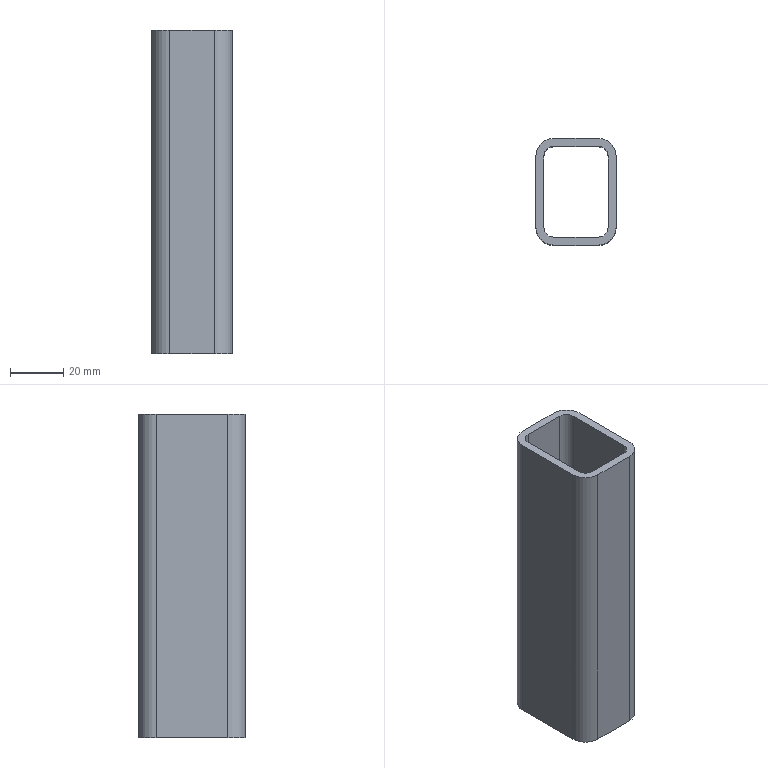Part | STEP file | DIN EN 10305-5 40 x 30 x 3 1785429634942 | 1 solid | 18 faces | box 30 x 40 x 121.4 mm | volume 43429 mm3 | plane 10 | cylinder 8 | commonest cylinder face diameters 7.2 x4 13.2 x4
STEP:
#1=CARTESIAN_POINT('',(-8.4,-17.,161.4));
#2=VERTEX_POINT('',#1);
#3=CARTESIAN_POINT('',(8.4,-17.,161.4));
#4=VERTEX_POINT('',#3);
#5=CARTESIAN_POINT('',(4.2,-17.,161.4));
#6=DIRECTION('',(1.,0.,0.));
#7=VECTOR('',#6,10.);
#8=LINE('',#5,#7);
#9=EDGE_CURVE('',#2,#4,#8,.T.);
#10=ORIENTED_EDGE('',*,*,#9,.T.);
#11=CARTESIAN_POINT('',(8.4,-17.,40.));
#12=VERTEX_POINT('',#11);
#13=CARTESIAN_POINT('',(8.4,-17.,0.));
#14=DIRECTION('',(0.,0.,1.));
#15=VECTOR('',#14,10.);
#16=LINE('',#13,#15);
#17=EDGE_CURVE('',#12,#4,#16,.T.);
#18=ORIENTED_EDGE('',*,*,#17,.F.);
#19=CARTESIAN_POINT('',(-8.4,-17.,40.));
#20=VERTEX_POINT('',#19);
#21=CARTESIAN_POINT('',(4.2,-17.,40.));
#22=DIRECTION('',(1.,0.,0.));
#23=VECTOR('',#22,10.);
#24=LINE('',#21,#23);
#25=EDGE_CURVE('',#20,#12,#24,.T.);
#26=ORIENTED_EDGE('',*,*,#25,.F.);
#27=CARTESIAN_POINT('',(-8.4,-17.,0.));
#28=DIRECTION('',(0.,0.,1.));
#29=VECTOR('',#28,10.);
#30=LINE('',#27,#29);
#31=EDGE_CURVE('',#20,#2,#30,.T.);
#32=ORIENTED_EDGE('',*,*,#31,.T.);
#33=EDGE_LOOP('',(#10,#18,#26,#32));
#34=FACE_OUTER_BOUND('',#33,.T.);
#35=CARTESIAN_POINT('',(8.4,-17.,0.));
#36=DIRECTION('',(0.,-1.,0.));
#37=DIRECTION('',(0.,0.,-1.));
#38=AXIS2_PLACEMENT_3D('',#35,#36,#37);
#39=PLANE('',#38);
#40=ADVANCED_FACE('',(#34),#39,.F.);
#41=CARTESIAN_POINT('',(12.,-13.4,161.4));
#42=VERTEX_POINT('',#41);
#43=CARTESIAN_POINT('',(8.4,-13.4,161.4));
#44=DIRECTION('',(0.,0.,1.));
#45=DIRECTION('',(0.,1.,0.));
#46=AXIS2_PLACEMENT_3D('',#43,#44,#45);
#47=CIRCLE('',#46,3.6);
#48=EDGE_CURVE('',#4,#42,#47,.T.);
#49=ORIENTED_EDGE('',*,*,#48,.T.);
#50=CARTESIAN_POINT('',(12.,-13.4,40.));
#51=VERTEX_POINT('',#50);
#52=CARTESIAN_POINT('',(12.,-13.4,0.));
#53=DIRECTION('',(0.,0.,1.));
#54=VECTOR('',#53,10.);
#55=LINE('',#52,#54);
#56=EDGE_CURVE('',#51,#42,#55,.T.);
#57=ORIENTED_EDGE('',*,*,#56,.F.);
#58=CARTESIAN_POINT('',(8.4,-13.4,40.));
#59=DIRECTION('',(0.,0.,1.));
#60=DIRECTION('',(0.,1.,0.));
#61=AXIS2_PLACEMENT_3D('',#58,#59,#60);
#62=CIRCLE('',#61,3.6);
#63=EDGE_CURVE('',#12,#51,#62,.T.);
#64=ORIENTED_EDGE('',*,*,#63,.F.);
#65=ORIENTED_EDGE('',*,*,#17,.T.);
#66=EDGE_LOOP('',(#49,#57,#64,#65));
#67=FACE_OUTER_BOUND('',#66,.T.);
#68=CARTESIAN_POINT('',(8.4,-13.4,0.));
#69=DIRECTION('',(0.,0.,1.));
#70=DIRECTION('',(0.,1.,0.));
#71=AXIS2_PLACEMENT_3D('',#68,#69,#70);
#72=CYLINDRICAL_SURFACE('',#71,3.6);
#73=ADVANCED_FACE('',(#67),#72,.F.);
#74=CARTESIAN_POINT('',(12.,13.4,161.4));
#75=VERTEX_POINT('',#74);
#76=CARTESIAN_POINT('',(12.,6.7,161.4));
#77=DIRECTION('',(0.,1.,0.));
#78=VECTOR('',#77,10.);
#79=LINE('',#76,#78);
#80=EDGE_CURVE('',#42,#75,#79,.T.);
#81=ORIENTED_EDGE('',*,*,#80,.T.);
#82=CARTESIAN_POINT('',(12.,13.4,40.));
#83=VERTEX_POINT('',#82);
#84=CARTESIAN_POINT('',(12.,13.4,0.));
#85=DIRECTION('',(0.,0.,1.));
#86=VECTOR('',#85,10.);
#87=LINE('',#84,#86);
#88=EDGE_CURVE('',#83,#75,#87,.T.);
#89=ORIENTED_EDGE('',*,*,#88,.F.);
#90=CARTESIAN_POINT('',(12.,6.7,40.));
#91=DIRECTION('',(0.,1.,0.));
#92=VECTOR('',#91,10.);
#93=LINE('',#90,#92);
#94=EDGE_CURVE('',#51,#83,#93,.T.);
#95=ORIENTED_EDGE('',*,*,#94,.F.);
#96=ORIENTED_EDGE('',*,*,#56,.T.);
#97=EDGE_LOOP('',(#81,#89,#95,#96));
#98=FACE_OUTER_BOUND('',#97,.T.);
#99=CARTESIAN_POINT('',(12.,13.4,0.));
#100=DIRECTION('',(1.,0.,0.));
#101=DIRECTION('',(0.,0.,-1.));
#102=AXIS2_PLACEMENT_3D('',#99,#100,#101);
#103=PLANE('',#102);
#104=ADVANCED_FACE('',(#98),#103,.F.);
#105=CARTESIAN_POINT('',(8.4,17.,161.4));
#106=VERTEX_POINT('',#105);
#107=CARTESIAN_POINT('',(8.4,13.4,161.4));
#108=DIRECTION('',(0.,0.,1.));
#109=DIRECTION('',(-1.,0.,0.));
#110=AXIS2_PLACEMENT_3D('',#107,#108,#109);
#111=CIRCLE('',#110,3.6);
#112=EDGE_CURVE('',#75,#106,#111,.T.);
#113=ORIENTED_EDGE('',*,*,#112,.T.);
#114=CARTESIAN_POINT('',(8.4,17.,40.));
#115=VERTEX_POINT('',#114);
#116=CARTESIAN_POINT('',(8.4,17.,0.));
#117=DIRECTION('',(0.,0.,1.));
#118=VECTOR('',#117,10.);
#119=LINE('',#116,#118);
#120=EDGE_CURVE('',#115,#106,#119,.T.);
#121=ORIENTED_EDGE('',*,*,#120,.F.);
#122=CARTESIAN_POINT('',(8.4,13.4,40.));
#123=DIRECTION('',(0.,0.,1.));
#124=DIRECTION('',(-1.,0.,0.));
#125=AXIS2_PLACEMENT_3D('',#122,#123,#124);
#126=CIRCLE('',#125,3.6);
#127=EDGE_CURVE('',#83,#115,#126,.T.);
#128=ORIENTED_EDGE('',*,*,#127,.F.);
#129=ORIENTED_EDGE('',*,*,#88,.T.);
#130=EDGE_LOOP('',(#113,#121,#128,#129));
#131=FACE_OUTER_BOUND('',#130,.T.);
#132=CARTESIAN_POINT('',(8.4,13.4,0.));
#133=DIRECTION('',(0.,0.,1.));
#134=DIRECTION('',(-1.,0.,0.));
#135=AXIS2_PLACEMENT_3D('',#132,#133,#134);
#136=CYLINDRICAL_SURFACE('',#135,3.6);
#137=ADVANCED_FACE('',(#131),#136,.F.);
#138=CARTESIAN_POINT('',(15.,13.4,161.4));
#139=VERTEX_POINT('',#138);
#140=CARTESIAN_POINT('',(15.,-13.4,161.4));
#141=VERTEX_POINT('',#140);
#142=CARTESIAN_POINT('',(15.,6.7,161.4));
#143=DIRECTION('',(0.,-1.,0.));
#144=VECTOR('',#143,10.);
#145=LINE('',#142,#144);
#146=EDGE_CURVE('',#139,#141,#145,.T.);
#147=ORIENTED_EDGE('',*,*,#146,.T.);
#148=CARTESIAN_POINT('',(15.,-13.4,40.));
#149=VERTEX_POINT('',#148);
#150=CARTESIAN_POINT('',(15.,-13.4,0.));
#151=DIRECTION('',(0.,0.,1.));
#152=VECTOR('',#151,10.);
#153=LINE('',#150,#152);
#154=EDGE_CURVE('',#149,#141,#153,.T.);
#155=ORIENTED_EDGE('',*,*,#154,.F.);
#156=CARTESIAN_POINT('',(15.,13.4,40.));
#157=VERTEX_POINT('',#156);
#158=CARTESIAN_POINT('',(15.,6.7,40.));
#159=DIRECTION('',(0.,-1.,0.));
#160=VECTOR('',#159,10.);
#161=LINE('',#158,#160);
#162=EDGE_CURVE('',#157,#149,#161,.T.);
#163=ORIENTED_EDGE('',*,*,#162,.F.);
#164=CARTESIAN_POINT('',(15.,13.4,0.));
#165=DIRECTION('',(0.,0.,1.));
#166=VECTOR('',#165,10.);
#167=LINE('',#164,#166);
#168=EDGE_CURVE('',#157,#139,#167,.T.);
#169=ORIENTED_EDGE('',*,*,#168,.T.);
#170=EDGE_LOOP('',(#147,#155,#163,#169));
#171=FACE_OUTER_BOUND('',#170,.T.);
#172=CARTESIAN_POINT('',(15.,13.4,0.));
#173=DIRECTION('',(1.,0.,0.));
#174=DIRECTION('',(0.,0.,-1.));
#175=AXIS2_PLACEMENT_3D('',#172,#173,#174);
#176=PLANE('',#175);
#177=ADVANCED_FACE('',(#171),#176,.T.);
#178=CARTESIAN_POINT('',(8.4,-20.,161.4));
#179=VERTEX_POINT('',#178);
#180=CARTESIAN_POINT('',(8.4,-13.4,161.4));
#181=DIRECTION('',(0.,0.,-1.));
#182=DIRECTION('',(0.,1.,0.));
#183=AXIS2_PLACEMENT_3D('',#180,#181,#182);
#184=CIRCLE('',#183,6.6);
#185=EDGE_CURVE('',#141,#179,#184,.T.);
#186=ORIENTED_EDGE('',*,*,#185,.T.);
#187=CARTESIAN_POINT('',(8.4,-20.,40.));
#188=VERTEX_POINT('',#187);
#189=CARTESIAN_POINT('',(8.4,-20.,0.));
#190=DIRECTION('',(0.,0.,1.));
#191=VECTOR('',#190,10.);
#192=LINE('',#189,#191);
#193=EDGE_CURVE('',#188,#179,#192,.T.);
#194=ORIENTED_EDGE('',*,*,#193,.F.);
#195=CARTESIAN_POINT('',(8.4,-13.4,40.));
#196=DIRECTION('',(0.,0.,-1.));
#197=DIRECTION('',(0.,1.,0.));
#198=AXIS2_PLACEMENT_3D('',#195,#196,#197);
#199=CIRCLE('',#198,6.6);
#200=EDGE_CURVE('',#149,#188,#199,.T.);
#201=ORIENTED_EDGE('',*,*,#200,.F.);
#202=ORIENTED_EDGE('',*,*,#154,.T.);
#203=EDGE_LOOP('',(#186,#194,#201,#202));
#204=FACE_OUTER_BOUND('',#203,.T.);
#205=CARTESIAN_POINT('',(8.4,-13.4,0.));
#206=DIRECTION('',(0.,0.,1.));
#207=DIRECTION('',(0.,1.,0.));
#208=AXIS2_PLACEMENT_3D('',#205,#206,#207);
#209=CYLINDRICAL_SURFACE('',#208,6.6);
#210=ADVANCED_FACE('',(#204),#209,.T.);
#211=CARTESIAN_POINT('',(-8.4,-20.,161.4));
#212=VERTEX_POINT('',#211);
#213=CARTESIAN_POINT('',(4.2,-20.,161.4));
#214=DIRECTION('',(-1.,0.,0.));
#215=VECTOR('',#214,10.);
#216=LINE('',#213,#215);
#217=EDGE_CURVE('',#179,#212,#216,.T.);
#218=ORIENTED_EDGE('',*,*,#217,.T.);
#219=CARTESIAN_POINT('',(-8.4,-20.,40.));
#220=VERTEX_POINT('',#219);
#221=CARTESIAN_POINT('',(-8.4,-20.,0.));
#222=DIRECTION('',(0.,0.,1.));
#223=VECTOR('',#222,10.);
#224=LINE('',#221,#223);
#225=EDGE_CURVE('',#220,#212,#224,.T.);
#226=ORIENTED_EDGE('',*,*,#225,.F.);
#227=CARTESIAN_POINT('',(4.2,-20.,40.));
#228=DIRECTION('',(-1.,0.,0.));
#229=VECTOR('',#228,10.);
#230=LINE('',#227,#229);
#231=EDGE_CURVE('',#188,#220,#230,.T.);
#232=ORIENTED_EDGE('',*,*,#231,.F.);
#233=ORIENTED_EDGE('',*,*,#193,.T.);
#234=EDGE_LOOP('',(#218,#226,#232,#233));
#235=FACE_OUTER_BOUND('',#234,.T.);
#236=CARTESIAN_POINT('',(8.4,-20.,0.));
#237=DIRECTION('',(0.,-1.,0.));
#238=DIRECTION('',(0.,0.,-1.));
#239=AXIS2_PLACEMENT_3D('',#236,#237,#238);
#240=PLANE('',#239);
#241=ADVANCED_FACE('',(#235),#240,.T.);
#242=CARTESIAN_POINT('',(-15.,-13.4,161.4));
#243=VERTEX_POINT('',#242);
#244=CARTESIAN_POINT('',(-8.4,-13.4,161.4));
#245=DIRECTION('',(0.,0.,-1.));
#246=DIRECTION('',(1.,0.,0.));
#247=AXIS2_PLACEMENT_3D('',#244,#245,#246);
#248=CIRCLE('',#247,6.6);
#249=EDGE_CURVE('',#212,#243,#248,.T.);
#250=ORIENTED_EDGE('',*,*,#249,.T.);
#251=CARTESIAN_POINT('',(-15.,-13.4,40.));
#252=VERTEX_POINT('',#251);
#253=CARTESIAN_POINT('',(-15.,-13.4,0.));
#254=DIRECTION('',(0.,0.,1.));
#255=VECTOR('',#254,10.);
#256=LINE('',#253,#255);
#257=EDGE_CURVE('',#252,#243,#256,.T.);
#258=ORIENTED_EDGE('',*,*,#257,.F.);
#259=CARTESIAN_POINT('',(-8.4,-13.4,40.));
#260=DIRECTION('',(0.,0.,-1.));
#261=DIRECTION('',(1.,0.,0.));
#262=AXIS2_PLACEMENT_3D('',#259,#260,#261);
#263=CIRCLE('',#262,6.6);
#264=EDGE_CURVE('',#220,#252,#263,.T.);
#265=ORIENTED_EDGE('',*,*,#264,.F.);
#266=ORIENTED_EDGE('',*,*,#225,.T.);
#267=EDGE_LOOP('',(#250,#258,#265,#266));
#268=FACE_OUTER_BOUND('',#267,.T.);
#269=CARTESIAN_POINT('',(-8.4,-13.4,0.));
#270=DIRECTION('',(0.,0.,1.));
#271=DIRECTION('',(1.,0.,0.));
#272=AXIS2_PLACEMENT_3D('',#269,#270,#271);
#273=CYLINDRICAL_SURFACE('',#272,6.6);
#274=ADVANCED_FACE('',(#268),#273,.T.);
#275=CARTESIAN_POINT('',(-8.4,17.,161.4));
#276=VERTEX_POINT('',#275);
#277=CARTESIAN_POINT('',(-4.2,17.,161.4));
#278=DIRECTION('',(-1.,0.,0.));
#279=VECTOR('',#278,10.);
#280=LINE('',#277,#279);
#281=EDGE_CURVE('',#106,#276,#280,.T.);
#282=ORIENTED_EDGE('',*,*,#281,.T.);
#283=CARTESIAN_POINT('',(-8.4,17.,40.));
#284=VERTEX_POINT('',#283);
#285=CARTESIAN_POINT('',(-8.4,17.,0.));
#286=DIRECTION('',(0.,0.,1.));
#287=VECTOR('',#286,10.);
#288=LINE('',#285,#287);
#289=EDGE_CURVE('',#284,#276,#288,.T.);
#290=ORIENTED_EDGE('',*,*,#289,.F.);
#291=CARTESIAN_POINT('',(-4.2,17.,40.));
#292=DIRECTION('',(-1.,0.,0.));
#293=VECTOR('',#292,10.);
#294=LINE('',#291,#293);
#295=EDGE_CURVE('',#115,#284,#294,.T.);
#296=ORIENTED_EDGE('',*,*,#295,.F.);
#297=ORIENTED_EDGE('',*,*,#120,.T.);
#298=EDGE_LOOP('',(#282,#290,#296,#297));
#299=FACE_OUTER_BOUND('',#298,.T.);
#300=CARTESIAN_POINT('',(-8.4,17.,0.));
#301=DIRECTION('',(0.,1.,0.));
#302=DIRECTION('',(0.,0.,1.));
#303=AXIS2_PLACEMENT_3D('',#300,#301,#302);
#304=PLANE('',#303);
#305=ADVANCED_FACE('',(#299),#304,.F.);
#306=CARTESIAN_POINT('',(-12.,-13.4,161.4));
#307=VERTEX_POINT('',#306);
#308=CARTESIAN_POINT('',(-8.4,-13.4,161.4));
#309=DIRECTION('',(0.,0.,1.));
#310=DIRECTION('',(1.,0.,0.));
#311=AXIS2_PLACEMENT_3D('',#308,#309,#310);
#312=CIRCLE('',#311,3.6);
#313=EDGE_CURVE('',#307,#2,#312,.T.);
#314=ORIENTED_EDGE('',*,*,#313,.T.);
#315=ORIENTED_EDGE('',*,*,#31,.F.);
#316=CARTESIAN_POINT('',(-12.,-13.4,40.));
#317=VERTEX_POINT('',#316);
#318=CARTESIAN_POINT('',(-8.4,-13.4,40.));
#319=DIRECTION('',(0.,0.,1.));
#320=DIRECTION('',(1.,0.,0.));
#321=AXIS2_PLACEMENT_3D('',#318,#319,#320);
#322=CIRCLE('',#321,3.6);
#323=EDGE_CURVE('',#317,#20,#322,.T.);
#324=ORIENTED_EDGE('',*,*,#323,.F.);
#325=CARTESIAN_POINT('',(-12.,-13.4,0.));
#326=DIRECTION('',(0.,0.,1.));
#327=VECTOR('',#326,10.);
#328=LINE('',#325,#327);
#329=EDGE_CURVE('',#317,#307,#328,.T.);
#330=ORIENTED_EDGE('',*,*,#329,.T.);
#331=EDGE_LOOP('',(#314,#315,#324,#330));
#332=FACE_OUTER_BOUND('',#331,.T.);
#333=CARTESIAN_POINT('',(-8.4,-13.4,0.));
#334=DIRECTION('',(0.,0.,1.));
#335=DIRECTION('',(1.,0.,0.));
#336=AXIS2_PLACEMENT_3D('',#333,#334,#335);
#337=CYLINDRICAL_SURFACE('',#336,3.6);
#338=ADVANCED_FACE('',(#332),#337,.F.);
#339=CARTESIAN_POINT('',(-12.,13.4,161.4));
#340=VERTEX_POINT('',#339);
#341=CARTESIAN_POINT('',(-12.,-6.7,161.4));
#342=DIRECTION('',(0.,-1.,0.));
#343=VECTOR('',#342,10.);
#344=LINE('',#341,#343);
#345=EDGE_CURVE('',#340,#307,#344,.T.);
#346=ORIENTED_EDGE('',*,*,#345,.T.);
#347=ORIENTED_EDGE('',*,*,#329,.F.);
#348=CARTESIAN_POINT('',(-12.,13.4,40.));
#349=VERTEX_POINT('',#348);
#350=CARTESIAN_POINT('',(-12.,-6.7,40.));
#351=DIRECTION('',(0.,-1.,0.));
#352=VECTOR('',#351,10.);
#353=LINE('',#350,#352);
#354=EDGE_CURVE('',#349,#317,#353,.T.);
#355=ORIENTED_EDGE('',*,*,#354,.F.);
#356=CARTESIAN_POINT('',(-12.,13.4,0.));
#357=DIRECTION('',(0.,0.,1.));
#358=VECTOR('',#357,10.);
#359=LINE('',#356,#358);
#360=EDGE_CURVE('',#349,#340,#359,.T.);
#361=ORIENTED_EDGE('',*,*,#360,.T.);
#362=EDGE_LOOP('',(#346,#347,#355,#361));
#363=FACE_OUTER_BOUND('',#362,.T.);
#364=CARTESIAN_POINT('',(-12.,-13.4,0.));
#365=DIRECTION('',(-1.,0.,0.));
#366=DIRECTION('',(0.,0.,1.));
#367=AXIS2_PLACEMENT_3D('',#364,#365,#366);
#368=PLANE('',#367);
#369=ADVANCED_FACE('',(#363),#368,.F.);
#370=CARTESIAN_POINT('',(-8.4,13.4,161.4));
#371=DIRECTION('',(0.,0.,1.));
#372=DIRECTION('',(0.,-1.,0.));
#373=AXIS2_PLACEMENT_3D('',#370,#371,#372);
#374=CIRCLE('',#373,3.6);
#375=EDGE_CURVE('',#276,#340,#374,.T.);
#376=ORIENTED_EDGE('',*,*,#375,.T.);
#377=ORIENTED_EDGE('',*,*,#360,.F.);
#378=CARTESIAN_POINT('',(-8.4,13.4,40.));
#379=DIRECTION('',(0.,0.,1.));
#380=DIRECTION('',(0.,-1.,0.));
#381=AXIS2_PLACEMENT_3D('',#378,#379,#380);
#382=CIRCLE('',#381,3.6);
#383=EDGE_CURVE('',#284,#349,#382,.T.);
#384=ORIENTED_EDGE('',*,*,#383,.F.);
#385=ORIENTED_EDGE('',*,*,#289,.T.);
#386=EDGE_LOOP('',(#376,#377,#384,#385));
#387=FACE_OUTER_BOUND('',#386,.T.);
#388=CARTESIAN_POINT('',(-8.4,13.4,0.));
#389=DIRECTION('',(0.,0.,1.));
#390=DIRECTION('',(0.,-1.,0.));
#391=AXIS2_PLACEMENT_3D('',#388,#389,#390);
#392=CYLINDRICAL_SURFACE('',#391,3.6);
#393=ADVANCED_FACE('',(#387),#392,.F.);
#394=CARTESIAN_POINT('',(-15.,13.4,161.4));
#395=VERTEX_POINT('',#394);
#396=CARTESIAN_POINT('',(-15.,-6.7,161.4));
#397=DIRECTION('',(0.,1.,0.));
#398=VECTOR('',#397,10.);
#399=LINE('',#396,#398);
#400=EDGE_CURVE('',#243,#395,#399,.T.);
#401=ORIENTED_EDGE('',*,*,#400,.T.);
#402=CARTESIAN_POINT('',(-15.,13.4,40.));
#403=VERTEX_POINT('',#402);
#404=CARTESIAN_POINT('',(-15.,13.4,0.));
#405=DIRECTION('',(0.,0.,1.));
#406=VECTOR('',#405,10.);
#407=LINE('',#404,#406);
#408=EDGE_CURVE('',#403,#395,#407,.T.);
#409=ORIENTED_EDGE('',*,*,#408,.F.);
#410=CARTESIAN_POINT('',(-15.,-6.7,40.));
#411=DIRECTION('',(0.,1.,0.));
#412=VECTOR('',#411,10.);
#413=LINE('',#410,#412);
#414=EDGE_CURVE('',#252,#403,#413,.T.);
#415=ORIENTED_EDGE('',*,*,#414,.F.);
#416=ORIENTED_EDGE('',*,*,#257,.T.);
#417=EDGE_LOOP('',(#401,#409,#415,#416));
#418=FACE_OUTER_BOUND('',#417,.T.);
#419=CARTESIAN_POINT('',(-15.,-13.4,0.));
#420=DIRECTION('',(-1.,0.,0.));
#421=DIRECTION('',(0.,0.,1.));
#422=AXIS2_PLACEMENT_3D('',#419,#420,#421);
#423=PLANE('',#422);
#424=ADVANCED_FACE('',(#418),#423,.T.);
#425=CARTESIAN_POINT('',(-8.4,20.,161.4));
#426=VERTEX_POINT('',#425);
#427=CARTESIAN_POINT('',(-8.4,13.4,161.4));
#428=DIRECTION('',(0.,0.,-1.));
#429=DIRECTION('',(0.,-1.,0.));
#430=AXIS2_PLACEMENT_3D('',#427,#428,#429);
#431=CIRCLE('',#430,6.6);
#432=EDGE_CURVE('',#395,#426,#431,.T.);
#433=ORIENTED_EDGE('',*,*,#432,.T.);
#434=CARTESIAN_POINT('',(-8.4,20.,40.));
#435=VERTEX_POINT('',#434);
#436=CARTESIAN_POINT('',(-8.4,20.,0.));
#437=DIRECTION('',(0.,0.,1.));
#438=VECTOR('',#437,10.);
#439=LINE('',#436,#438);
#440=EDGE_CURVE('',#435,#426,#439,.T.);
#441=ORIENTED_EDGE('',*,*,#440,.F.);
#442=CARTESIAN_POINT('',(-8.4,13.4,40.));
#443=DIRECTION('',(0.,0.,-1.));
#444=DIRECTION('',(0.,-1.,0.));
#445=AXIS2_PLACEMENT_3D('',#442,#443,#444);
#446=CIRCLE('',#445,6.6);
#447=EDGE_CURVE('',#403,#435,#446,.T.);
#448=ORIENTED_EDGE('',*,*,#447,.F.);
#449=ORIENTED_EDGE('',*,*,#408,.T.);
#450=EDGE_LOOP('',(#433,#441,#448,#449));
#451=FACE_OUTER_BOUND('',#450,.T.);
#452=CARTESIAN_POINT('',(-8.4,13.4,0.));
#453=DIRECTION('',(0.,0.,1.));
#454=DIRECTION('',(0.,-1.,0.));
#455=AXIS2_PLACEMENT_3D('',#452,#453,#454);
#456=CYLINDRICAL_SURFACE('',#455,6.6);
#457=ADVANCED_FACE('',(#451),#456,.T.);
#458=CARTESIAN_POINT('',(8.4,20.,161.4));
#459=VERTEX_POINT('',#458);
#460=CARTESIAN_POINT('',(-4.2,20.,161.4));
#461=DIRECTION('',(1.,0.,0.));
#462=VECTOR('',#461,10.);
#463=LINE('',#460,#462);
#464=EDGE_CURVE('',#426,#459,#463,.T.);
#465=ORIENTED_EDGE('',*,*,#464,.T.);
#466=CARTESIAN_POINT('',(8.4,20.,40.));
#467=VERTEX_POINT('',#466);
#468=CARTESIAN_POINT('',(8.4,20.,0.));
#469=DIRECTION('',(0.,0.,1.));
#470=VECTOR('',#469,10.);
#471=LINE('',#468,#470);
#472=EDGE_CURVE('',#467,#459,#471,.T.);
#473=ORIENTED_EDGE('',*,*,#472,.F.);
#474=CARTESIAN_POINT('',(-4.2,20.,40.));
#475=DIRECTION('',(1.,0.,0.));
#476=VECTOR('',#475,10.);
#477=LINE('',#474,#476);
#478=EDGE_CURVE('',#435,#467,#477,.T.);
#479=ORIENTED_EDGE('',*,*,#478,.F.);
#480=ORIENTED_EDGE('',*,*,#440,.T.);
#481=EDGE_LOOP('',(#465,#473,#479,#480));
#482=FACE_OUTER_BOUND('',#481,.T.);
#483=CARTESIAN_POINT('',(-8.4,20.,0.));
#484=DIRECTION('',(0.,1.,0.));
#485=DIRECTION('',(0.,0.,1.));
#486=AXIS2_PLACEMENT_3D('',#483,#484,#485);
#487=PLANE('',#486);
#488=ADVANCED_FACE('',(#482),#487,.T.);
#489=CARTESIAN_POINT('',(8.4,13.4,161.4));
#490=DIRECTION('',(0.,0.,-1.));
#491=DIRECTION('',(-1.,0.,0.));
#492=AXIS2_PLACEMENT_3D('',#489,#490,#491);
#493=CIRCLE('',#492,6.6);
#494=EDGE_CURVE('',#459,#139,#493,.T.);
#495=ORIENTED_EDGE('',*,*,#494,.T.);
#496=ORIENTED_EDGE('',*,*,#168,.F.);
#497=CARTESIAN_POINT('',(8.4,13.4,40.));
#498=DIRECTION('',(0.,0.,-1.));
#499=DIRECTION('',(-1.,0.,0.));
#500=AXIS2_PLACEMENT_3D('',#497,#498,#499);
#501=CIRCLE('',#500,6.6);
#502=EDGE_CURVE('',#467,#157,#501,.T.);
#503=ORIENTED_EDGE('',*,*,#502,.F.);
#504=ORIENTED_EDGE('',*,*,#472,.T.);
#505=EDGE_LOOP('',(#495,#496,#503,#504));
#506=FACE_OUTER_BOUND('',#505,.T.);
#507=CARTESIAN_POINT('',(8.4,13.4,0.));
#508=DIRECTION('',(0.,0.,1.));
#509=DIRECTION('',(-1.,0.,0.));
#510=AXIS2_PLACEMENT_3D('',#507,#508,#509);
#511=CYLINDRICAL_SURFACE('',#510,6.6);
#512=ADVANCED_FACE('',(#506),#511,.T.);
#513=ORIENTED_EDGE('',*,*,#414,.T.);
#514=ORIENTED_EDGE('',*,*,#447,.T.);
#515=ORIENTED_EDGE('',*,*,#478,.T.);
#516=ORIENTED_EDGE('',*,*,#502,.T.);
#517=ORIENTED_EDGE('',*,*,#162,.T.);
#518=ORIENTED_EDGE('',*,*,#200,.T.);
#519=ORIENTED_EDGE('',*,*,#231,.T.);
#520=ORIENTED_EDGE('',*,*,#264,.T.);
#521=EDGE_LOOP('',(#513,#514,#515,#516,#517,#518,#519,#520));
#522=FACE_OUTER_BOUND('',#521,.T.);
#523=ORIENTED_EDGE('',*,*,#295,.T.);
#524=ORIENTED_EDGE('',*,*,#383,.T.);
#525=ORIENTED_EDGE('',*,*,#354,.T.);
#526=ORIENTED_EDGE('',*,*,#323,.T.);
#527=ORIENTED_EDGE('',*,*,#25,.T.);
#528=ORIENTED_EDGE('',*,*,#63,.T.);
#529=ORIENTED_EDGE('',*,*,#94,.T.);
#530=ORIENTED_EDGE('',*,*,#127,.T.);
#531=EDGE_LOOP('',(#523,#524,#525,#526,#527,#528,#529,#530));
#532=FACE_BOUND('',#531,.T.);
#533=CARTESIAN_POINT('',(0.,0.,40.));
#534=DIRECTION('',(0.,0.,1.));
#535=DIRECTION('',(1.,0.,0.));
#536=AXIS2_PLACEMENT_3D('',#533,#534,#535);
#537=PLANE('',#536);
#538=ADVANCED_FACE('',(#522,#532),#537,.F.);
#539=ORIENTED_EDGE('',*,*,#400,.F.);
#540=ORIENTED_EDGE('',*,*,#249,.F.);
#541=ORIENTED_EDGE('',*,*,#217,.F.);
#542=ORIENTED_EDGE('',*,*,#185,.F.);
#543=ORIENTED_EDGE('',*,*,#146,.F.);
#544=ORIENTED_EDGE('',*,*,#494,.F.);
#545=ORIENTED_EDGE('',*,*,#464,.F.);
#546=ORIENTED_EDGE('',*,*,#432,.F.);
#547=EDGE_LOOP('',(#539,#540,#541,#542,#543,#544,#545,#546));
#548=FACE_OUTER_BOUND('',#547,.T.);
#549=ORIENTED_EDGE('',*,*,#281,.F.);
#550=ORIENTED_EDGE('',*,*,#112,.F.);
#551=ORIENTED_EDGE('',*,*,#80,.F.);
#552=ORIENTED_EDGE('',*,*,#48,.F.);
#553=ORIENTED_EDGE('',*,*,#9,.F.);
#554=ORIENTED_EDGE('',*,*,#313,.F.);
#555=ORIENTED_EDGE('',*,*,#345,.F.);
#556=ORIENTED_EDGE('',*,*,#375,.F.);
#557=EDGE_LOOP('',(#549,#550,#551,#552,#553,#554,#555,#556));
#558=FACE_BOUND('',#557,.T.);
#559=CARTESIAN_POINT('',(0.,0.,161.4));
#560=DIRECTION('',(0.,0.,1.));
#561=DIRECTION('',(1.,0.,0.));
#562=AXIS2_PLACEMENT_3D('',#559,#560,#561);
#563=PLANE('',#562);
#564=ADVANCED_FACE('',(#548,#558),#563,.T.);
#565=CLOSED_SHELL('',(#40,#73,#104,#137,#177,#210,#241,#274,#305,#338,#369,#393,#424,#457,#488,#512,#538,#564));
#566=MANIFOLD_SOLID_BREP('',#565);
#567=(LENGTH_UNIT()NAMED_UNIT(*)SI_UNIT(.MILLI.,.METRE.));
#568=UNCERTAINTY_MEASURE_WITH_UNIT(LENGTH_MEASURE(0.01),#567,'','');
#569=(NAMED_UNIT(*)PLANE_ANGLE_UNIT()SI_UNIT($,.RADIAN.));
#570=(NAMED_UNIT(*)SI_UNIT($,.STERADIAN.)SOLID_ANGLE_UNIT());
#571=(GEOMETRIC_REPRESENTATION_CONTEXT(3)GLOBAL_UNCERTAINTY_ASSIGNED_CONTEXT((#568))GLOBAL_UNIT_ASSIGNED_CONTEXT((#567,#569,#570))REPRESENTATION_CONTEXT('',''));
#572=ADVANCED_BREP_SHAPE_REPRESENTATION('',(#566),#571);